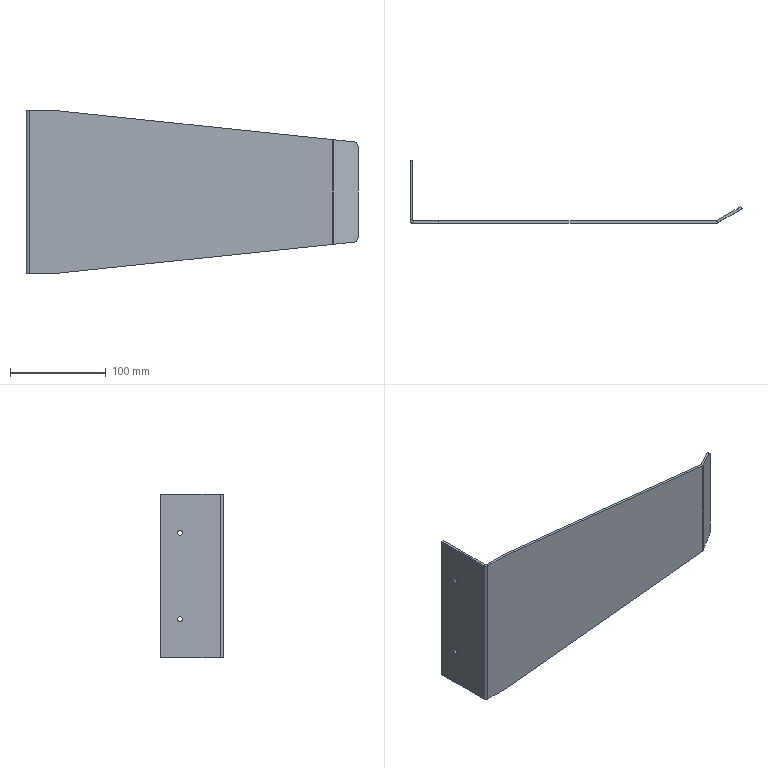Part | SolidWorks | features Fillet 1, FlatPattern 1, HoleWzd 1, ICE 1, MirrorPattern 1, SMBaseFlange 1, SheetMetal 1 | 1 solid | 30 faces | box 345.981 x 65 x 170 mm | volume 147766 mm3 | plane 18 | cylinder 10 | spline 2 | commonest cylinder face diameters 5 x4 1.473 x2 6.473 x2 10 x2
STEP:
#1=CARTESIAN_POINT('',(0.,45.,47.5));
#2=VERTEX_POINT('',#1);
#3=CARTESIAN_POINT('',(0.,45.,42.5));
#4=VERTEX_POINT('',#3);
#5=CARTESIAN_POINT('',(0.,45.,45.));
#6=DIRECTION('',(1.,0.,0.));
#7=DIRECTION('',(0.,0.,-1.));
#8=AXIS2_PLACEMENT_3D('',#5,#6,#7);
#9=CIRCLE('',#8,2.5);
#10=EDGE_CURVE('',#2,#4,#9,.T.);
#11=ORIENTED_EDGE('',*,*,#10,.F.);
#12=CARTESIAN_POINT('',(2.5,45.,47.5));
#13=VERTEX_POINT('',#12);
#14=CARTESIAN_POINT('',(2.5,45.,47.5));
#15=DIRECTION('',(1.,0.,0.));
#16=VECTOR('',#15,1000.);
#17=LINE('',#14,#16);
#18=EDGE_CURVE('',#2,#13,#17,.T.);
#19=ORIENTED_EDGE('',*,*,#18,.T.);
#20=CARTESIAN_POINT('',(2.5,45.,42.5));
#21=VERTEX_POINT('',#20);
#22=CARTESIAN_POINT('',(2.5,45.,45.));
#23=DIRECTION('',(1.,0.,0.));
#24=DIRECTION('',(0.,0.,-1.));
#25=AXIS2_PLACEMENT_3D('',#22,#23,#24);
#26=CIRCLE('',#25,2.5);
#27=EDGE_CURVE('',#13,#21,#26,.T.);
#28=ORIENTED_EDGE('',*,*,#27,.T.);
#29=CARTESIAN_POINT('',(2.5,45.,42.5));
#30=DIRECTION('',(1.,0.,0.));
#31=VECTOR('',#30,1000.);
#32=LINE('',#29,#31);
#33=EDGE_CURVE('',#4,#21,#32,.T.);
#34=ORIENTED_EDGE('',*,*,#33,.F.);
#35=EDGE_LOOP('',(#11,#19,#28,#34));
#36=FACE_OUTER_BOUND('',#35,.T.);
#37=CARTESIAN_POINT('',(2.5,45.,45.));
#38=DIRECTION('',(1.,0.,0.));
#39=DIRECTION('',(0.,0.,-1.));
#40=AXIS2_PLACEMENT_3D('',#37,#38,#39);
#41=CYLINDRICAL_SURFACE('',#40,2.5);
#42=ADVANCED_FACE('',(#36),#41,.F.);
#43=CARTESIAN_POINT('',(0.,45.,-42.5));
#44=VERTEX_POINT('',#43);
#45=CARTESIAN_POINT('',(0.,45.,-47.5));
#46=VERTEX_POINT('',#45);
#47=CARTESIAN_POINT('',(0.,45.,-45.));
#48=DIRECTION('',(1.,0.,0.));
#49=DIRECTION('',(0.,0.,-1.));
#50=AXIS2_PLACEMENT_3D('',#47,#48,#49);
#51=CIRCLE('',#50,2.5);
#52=EDGE_CURVE('',#44,#46,#51,.T.);
#53=ORIENTED_EDGE('',*,*,#52,.F.);
#54=CARTESIAN_POINT('',(2.5,45.,-42.5));
#55=VERTEX_POINT('',#54);
#56=CARTESIAN_POINT('',(2.5,45.,-42.5));
#57=DIRECTION('',(1.,0.,0.));
#58=VECTOR('',#57,1000.);
#59=LINE('',#56,#58);
#60=EDGE_CURVE('',#44,#55,#59,.T.);
#61=ORIENTED_EDGE('',*,*,#60,.T.);
#62=CARTESIAN_POINT('',(2.5,45.,-47.5));
#63=VERTEX_POINT('',#62);
#64=CARTESIAN_POINT('',(2.5,45.,-45.));
#65=DIRECTION('',(1.,0.,0.));
#66=DIRECTION('',(0.,0.,-1.));
#67=AXIS2_PLACEMENT_3D('',#64,#65,#66);
#68=CIRCLE('',#67,2.5);
#69=EDGE_CURVE('',#55,#63,#68,.T.);
#70=ORIENTED_EDGE('',*,*,#69,.T.);
#71=CARTESIAN_POINT('',(2.5,45.,-47.5));
#72=DIRECTION('',(1.,0.,0.));
#73=VECTOR('',#72,1000.);
#74=LINE('',#71,#73);
#75=EDGE_CURVE('',#46,#63,#74,.T.);
#76=ORIENTED_EDGE('',*,*,#75,.F.);
#77=EDGE_LOOP('',(#53,#61,#70,#76));
#78=FACE_OUTER_BOUND('',#77,.T.);
#79=CARTESIAN_POINT('',(2.5,45.,-45.));
#80=DIRECTION('',(1.,0.,0.));
#81=DIRECTION('',(0.,0.,-1.));
#82=AXIS2_PLACEMENT_3D('',#79,#80,#81);
#83=CYLINDRICAL_SURFACE('',#82,2.5);
#84=ADVANCED_FACE('',(#78),#83,.F.);
#85=CARTESIAN_POINT('',(320.751,0.4336,-54.441));
#86=VERTEX_POINT('',#85);
#87=CARTESIAN_POINT('',(342.043,12.727,-52.203));
#88=VERTEX_POINT('',#87);
#89=CARTESIAN_POINT('',(330.908,6.298,-53.373));
#90=DIRECTION('',(0.8625,0.4979,0.09065));
#91=VECTOR('',#90,1000.);
#92=LINE('',#89,#91);
#93=EDGE_CURVE('',#86,#88,#92,.T.);
#94=ORIENTED_EDGE('',*,*,#93,.T.);
#95=CARTESIAN_POINT('',(345.981,15.,-47.224));
#96=VERTEX_POINT('',#95);
#97=CARTESIAN_POINT('',(341.651,12.5,-47.224));
#98=DIRECTION('',(0.5,-0.866,0.));
#99=DIRECTION('',(-0.866,-0.5,0.));
#100=AXIS2_PLACEMENT_3D('',#97,#98,#99);
#101=CIRCLE('',#100,5.);
#102=EDGE_CURVE('',#88,#96,#101,.T.);
#103=ORIENTED_EDGE('',*,*,#102,.T.);
#104=CARTESIAN_POINT('',(345.981,15.,47.224));
#105=VERTEX_POINT('',#104);
#106=CARTESIAN_POINT('',(345.981,15.,85.));
#107=DIRECTION('',(0.,0.,-1.));
#108=VECTOR('',#107,1000.);
#109=LINE('',#106,#108);
#110=EDGE_CURVE('',#105,#96,#109,.T.);
#111=ORIENTED_EDGE('',*,*,#110,.F.);
#112=CARTESIAN_POINT('',(342.043,12.727,52.203));
#113=VERTEX_POINT('',#112);
#114=CARTESIAN_POINT('',(341.651,12.5,47.224));
#115=DIRECTION('',(0.5,-0.866,0.));
#116=DIRECTION('',(-0.866,-0.5,0.));
#117=AXIS2_PLACEMENT_3D('',#114,#115,#116);
#118=CIRCLE('',#117,5.);
#119=EDGE_CURVE('',#105,#113,#118,.T.);
#120=ORIENTED_EDGE('',*,*,#119,.T.);
#121=CARTESIAN_POINT('',(320.751,0.4336,54.441));
#122=VERTEX_POINT('',#121);
#123=CARTESIAN_POINT('',(317.617,-1.376,54.77));
#124=DIRECTION('',(0.8625,0.4979,-0.09065));
#125=VECTOR('',#124,1000.);
#126=LINE('',#123,#125);
#127=EDGE_CURVE('',#122,#113,#126,.T.);
#128=ORIENTED_EDGE('',*,*,#127,.F.);
#129=CARTESIAN_POINT('',(320.751,0.4336,85.));
#130=DIRECTION('',(0.,0.,-1.));
#131=VECTOR('',#130,1000.);
#132=LINE('',#129,#131);
#133=EDGE_CURVE('',#122,#86,#132,.T.);
#134=ORIENTED_EDGE('',*,*,#133,.T.);
#135=EDGE_LOOP('',(#94,#103,#111,#120,#128,#134));
#136=FACE_OUTER_BOUND('',#135,.T.);
#137=CARTESIAN_POINT('',(320.,0.,85.));
#138=DIRECTION('',(-0.5,0.866,0.));
#139=DIRECTION('',(-0.866,-0.5,0.));
#140=AXIS2_PLACEMENT_3D('',#137,#138,#139);
#141=PLANE('',#140);
#142=ADVANCED_FACE('',(#136),#141,.F.);
#143=ORIENTED_EDGE('',*,*,#110,.T.);
#144=CARTESIAN_POINT('',(344.731,17.165,-47.224));
#145=VERTEX_POINT('',#144);
#146=CARTESIAN_POINT('',(344.731,17.165,-47.224));
#147=DIRECTION('',(-0.5,0.866,0.));
#148=VECTOR('',#147,1000.);
#149=LINE('',#146,#148);
#150=EDGE_CURVE('',#96,#145,#149,.T.);
#151=ORIENTED_EDGE('',*,*,#150,.T.);
#152=CARTESIAN_POINT('',(344.731,17.165,47.224));
#153=VERTEX_POINT('',#152);
#154=CARTESIAN_POINT('',(344.731,17.165,85.));
#155=DIRECTION('',(0.,0.,-1.));
#156=VECTOR('',#155,1000.);
#157=LINE('',#154,#156);
#158=EDGE_CURVE('',#153,#145,#157,.T.);
#159=ORIENTED_EDGE('',*,*,#158,.F.);
#160=CARTESIAN_POINT('',(344.731,17.165,47.224));
#161=DIRECTION('',(0.5,-0.866,0.));
#162=VECTOR('',#161,1000.);
#163=LINE('',#160,#162);
#164=EDGE_CURVE('',#153,#105,#163,.T.);
#165=ORIENTED_EDGE('',*,*,#164,.T.);
#166=EDGE_LOOP('',(#143,#151,#159,#165));
#167=FACE_OUTER_BOUND('',#166,.T.);
#168=CARTESIAN_POINT('',(344.731,17.165,85.));
#169=DIRECTION('',(0.866,0.5,0.));
#170=DIRECTION('',(-0.5,0.866,0.));
#171=AXIS2_PLACEMENT_3D('',#168,#169,#170);
#172=PLANE('',#171);
#173=ADVANCED_FACE('',(#167),#172,.T.);
#174=ORIENTED_EDGE('',*,*,#158,.T.);
#175=CARTESIAN_POINT('',(340.793,14.892,-52.203));
#176=VERTEX_POINT('',#175);
#177=CARTESIAN_POINT('',(340.401,14.665,-47.224));
#178=DIRECTION('',(-0.5,0.866,0.));
#179=DIRECTION('',(-0.866,-0.5,0.));
#180=AXIS2_PLACEMENT_3D('',#177,#178,#179);
#181=CIRCLE('',#180,5.);
#182=EDGE_CURVE('',#145,#176,#181,.T.);
#183=ORIENTED_EDGE('',*,*,#182,.T.);
#184=CARTESIAN_POINT('',(319.501,2.599,-54.441));
#185=VERTEX_POINT('',#184);
#186=CARTESIAN_POINT('',(329.658,8.463,-53.373));
#187=DIRECTION('',(0.8625,0.4979,0.09065));
#188=VECTOR('',#187,1000.);
#189=LINE('',#186,#188);
#190=EDGE_CURVE('',#185,#176,#189,.T.);
#191=ORIENTED_EDGE('',*,*,#190,.F.);
#192=CARTESIAN_POINT('',(319.501,2.599,54.441));
#193=VERTEX_POINT('',#192);
#194=CARTESIAN_POINT('',(319.501,2.599,85.));
#195=DIRECTION('',(0.,0.,-1.));
#196=VECTOR('',#195,1000.);
#197=LINE('',#194,#196);
#198=EDGE_CURVE('',#193,#185,#197,.T.);
#199=ORIENTED_EDGE('',*,*,#198,.F.);
#200=CARTESIAN_POINT('',(340.793,14.892,52.203));
#201=VERTEX_POINT('',#200);
#202=CARTESIAN_POINT('',(316.367,0.7893,54.77));
#203=DIRECTION('',(0.8625,0.4979,-0.09065));
#204=VECTOR('',#203,1000.);
#205=LINE('',#202,#204);
#206=EDGE_CURVE('',#193,#201,#205,.T.);
#207=ORIENTED_EDGE('',*,*,#206,.T.);
#208=CARTESIAN_POINT('',(340.401,14.665,47.224));
#209=DIRECTION('',(-0.5,0.866,0.));
#210=DIRECTION('',(-0.866,-0.5,0.));
#211=AXIS2_PLACEMENT_3D('',#208,#209,#210);
#212=CIRCLE('',#211,5.);
#213=EDGE_CURVE('',#201,#153,#212,.T.);
#214=ORIENTED_EDGE('',*,*,#213,.T.);
#215=EDGE_LOOP('',(#174,#183,#191,#199,#207,#214));
#216=FACE_OUTER_BOUND('',#215,.T.);
#217=CARTESIAN_POINT('',(318.75,2.165,85.));
#218=DIRECTION('',(-0.5,0.866,0.));
#219=DIRECTION('',(-0.866,-0.5,0.));
#220=AXIS2_PLACEMENT_3D('',#217,#218,#219);
#221=PLANE('',#220);
#222=ADVANCED_FACE('',(#216),#221,.T.);
#223=CARTESIAN_POINT('',(319.133,2.5,54.611));
#224=VERTEX_POINT('',#223);
#225=CARTESIAN_POINT('',(319.133,2.5,-54.611));
#226=VERTEX_POINT('',#225);
#227=CARTESIAN_POINT('',(319.133,2.5,85.));
#228=DIRECTION('',(0.,0.,-1.));
#229=VECTOR('',#228,1000.);
#230=LINE('',#227,#229);
#231=EDGE_CURVE('',#224,#226,#230,.T.);
#232=ORIENTED_EDGE('',*,*,#231,.F.);
#233=CARTESIAN_POINT('',(319.133,2.5,54.611));
#234=CARTESIAN_POINT('',(319.263,2.5,54.551));
#235=CARTESIAN_POINT('',(319.388,2.534,54.493));
#236=CARTESIAN_POINT('',(319.501,2.599,54.441));
#237=(BOUNDED_CURVE()B_SPLINE_CURVE(3,(#233,#234,#235,#236),.UNSPECIFIED.,.F.,.T.)B_SPLINE_CURVE_WITH_KNOTS((4,4),(4.712,5.236),.UNSPECIFIED.)CURVE()GEOMETRIC_REPRESENTATION_ITEM()RATIONAL_B_SPLINE_CURVE((1.,0.9773,0.9773,1.))REPRESENTATION_ITEM(''));
#238=EDGE_CURVE('',#224,#193,#237,.T.);
#239=ORIENTED_EDGE('',*,*,#238,.T.);
#240=ORIENTED_EDGE('',*,*,#198,.T.);
#241=CARTESIAN_POINT('',(319.133,2.5,-54.611));
#242=CARTESIAN_POINT('',(319.263,2.5,-54.551));
#243=CARTESIAN_POINT('',(319.388,2.534,-54.493));
#244=CARTESIAN_POINT('',(319.501,2.599,-54.441));
#245=(BOUNDED_CURVE()B_SPLINE_CURVE(3,(#241,#242,#243,#244),.UNSPECIFIED.,.F.,.T.)B_SPLINE_CURVE_WITH_KNOTS((4,4),(1.571,2.094),.UNSPECIFIED.)CURVE()GEOMETRIC_REPRESENTATION_ITEM()RATIONAL_B_SPLINE_CURVE((1.,0.9773,0.9773,1.))REPRESENTATION_ITEM(''));
#246=EDGE_CURVE('',#226,#185,#245,.T.);
#247=ORIENTED_EDGE('',*,*,#246,.F.);
#248=EDGE_LOOP('',(#232,#239,#240,#247));
#249=FACE_OUTER_BOUND('',#248,.T.);
#250=CARTESIAN_POINT('',(319.133,3.237,85.));
#251=DIRECTION('',(0.,0.,-1.));
#252=DIRECTION('',(-1.,0.,0.));
#253=AXIS2_PLACEMENT_3D('',#250,#251,#252);
#254=CYLINDRICAL_SURFACE('',#253,0.7366);
#255=ADVANCED_FACE('',(#249),#254,.F.);
#256=CARTESIAN_POINT('',(3.237,2.5,85.));
#257=VERTEX_POINT('',#256);
#258=CARTESIAN_POINT('',(30.,2.5,85.));
#259=VERTEX_POINT('',#258);
#260=CARTESIAN_POINT('',(0.,2.5,85.));
#261=DIRECTION('',(1.,0.,0.));
#262=VECTOR('',#261,1000.);
#263=LINE('',#260,#262);
#264=EDGE_CURVE('',#257,#259,#263,.T.);
#265=ORIENTED_EDGE('',*,*,#264,.T.);
#266=CARTESIAN_POINT('',(0.3278,2.5,88.119));
#267=DIRECTION('',(0.9945,0.,-0.1045));
#268=VECTOR('',#267,1000.);
#269=LINE('',#266,#268);
#270=EDGE_CURVE('',#259,#224,#269,.T.);
#271=ORIENTED_EDGE('',*,*,#270,.T.);
#272=ORIENTED_EDGE('',*,*,#231,.T.);
#273=CARTESIAN_POINT('',(30.,2.5,-85.));
#274=VERTEX_POINT('',#273);
#275=CARTESIAN_POINT('',(18.,2.5,-86.261));
#276=DIRECTION('',(0.9945,0.,0.1045));
#277=VECTOR('',#276,1000.);
#278=LINE('',#275,#277);
#279=EDGE_CURVE('',#274,#226,#278,.T.);
#280=ORIENTED_EDGE('',*,*,#279,.F.);
#281=CARTESIAN_POINT('',(3.237,2.5,-85.));
#282=VERTEX_POINT('',#281);
#283=CARTESIAN_POINT('',(0.,2.5,-85.));
#284=DIRECTION('',(1.,0.,0.));
#285=VECTOR('',#284,1000.);
#286=LINE('',#283,#285);
#287=EDGE_CURVE('',#282,#274,#286,.T.);
#288=ORIENTED_EDGE('',*,*,#287,.F.);
#289=CARTESIAN_POINT('',(3.237,2.5,85.));
#290=DIRECTION('',(0.,0.,-1.));
#291=VECTOR('',#290,1000.);
#292=LINE('',#289,#291);
#293=EDGE_CURVE('',#257,#282,#292,.T.);
#294=ORIENTED_EDGE('',*,*,#293,.F.);
#295=EDGE_LOOP('',(#265,#271,#272,#280,#288,#294));
#296=FACE_OUTER_BOUND('',#295,.T.);
#297=CARTESIAN_POINT('',(0.,2.5,85.));
#298=DIRECTION('',(0.,1.,0.));
#299=DIRECTION('',(0.,0.,1.));
#300=AXIS2_PLACEMENT_3D('',#297,#298,#299);
#301=PLANE('',#300);
#302=ADVANCED_FACE('',(#296),#301,.T.);
#303=CARTESIAN_POINT('',(30.,0.,85.));
#304=VERTEX_POINT('',#303);
#305=CARTESIAN_POINT('',(319.133,0.,54.611));
#306=VERTEX_POINT('',#305);
#307=CARTESIAN_POINT('',(0.3278,0.,88.119));
#308=DIRECTION('',(0.9945,0.,-0.1045));
#309=VECTOR('',#308,1000.);
#310=LINE('',#307,#309);
#311=EDGE_CURVE('',#304,#306,#310,.T.);
#312=ORIENTED_EDGE('',*,*,#311,.F.);
#313=CARTESIAN_POINT('',(3.237,0.,85.));
#314=VERTEX_POINT('',#313);
#315=CARTESIAN_POINT('',(0.,0.,85.));
#316=DIRECTION('',(1.,0.,0.));
#317=VECTOR('',#316,1000.);
#318=LINE('',#315,#317);
#319=EDGE_CURVE('',#314,#304,#318,.T.);
#320=ORIENTED_EDGE('',*,*,#319,.F.);
#321=CARTESIAN_POINT('',(3.237,0.,-85.));
#322=VERTEX_POINT('',#321);
#323=CARTESIAN_POINT('',(3.237,0.,85.));
#324=DIRECTION('',(0.,0.,-1.));
#325=VECTOR('',#324,1000.);
#326=LINE('',#323,#325);
#327=EDGE_CURVE('',#314,#322,#326,.T.);
#328=ORIENTED_EDGE('',*,*,#327,.T.);
#329=CARTESIAN_POINT('',(30.,0.,-85.));
#330=VERTEX_POINT('',#329);
#331=CARTESIAN_POINT('',(0.,0.,-85.));
#332=DIRECTION('',(1.,0.,0.));
#333=VECTOR('',#332,1000.);
#334=LINE('',#331,#333);
#335=EDGE_CURVE('',#322,#330,#334,.T.);
#336=ORIENTED_EDGE('',*,*,#335,.T.);
#337=CARTESIAN_POINT('',(319.133,0.,-54.611));
#338=VERTEX_POINT('',#337);
#339=CARTESIAN_POINT('',(18.,0.,-86.261));
#340=DIRECTION('',(0.9945,0.,0.1045));
#341=VECTOR('',#340,1000.);
#342=LINE('',#339,#341);
#343=EDGE_CURVE('',#330,#338,#342,.T.);
#344=ORIENTED_EDGE('',*,*,#343,.T.);
#345=CARTESIAN_POINT('',(319.133,0.,85.));
#346=DIRECTION('',(0.,0.,-1.));
#347=VECTOR('',#346,1000.);
#348=LINE('',#345,#347);
#349=EDGE_CURVE('',#306,#338,#348,.T.);
#350=ORIENTED_EDGE('',*,*,#349,.F.);
#351=EDGE_LOOP('',(#312,#320,#328,#336,#344,#350));
#352=FACE_OUTER_BOUND('',#351,.T.);
#353=CARTESIAN_POINT('',(0.,0.,85.));
#354=DIRECTION('',(0.,1.,0.));
#355=DIRECTION('',(0.,0.,1.));
#356=AXIS2_PLACEMENT_3D('',#353,#354,#355);
#357=PLANE('',#356);
#358=ADVANCED_FACE('',(#352),#357,.F.);
#359=CARTESIAN_POINT('',(319.133,0.,54.611));
#360=CARTESIAN_POINT('',(319.704,0.,54.551));
#361=CARTESIAN_POINT('',(320.256,0.1479,54.493));
#362=CARTESIAN_POINT('',(320.751,0.4336,54.441));
#363=(BOUNDED_CURVE()B_SPLINE_CURVE(3,(#359,#360,#361,#362),.UNSPECIFIED.,.F.,.F.)B_SPLINE_CURVE_WITH_KNOTS((4,4),(4.712,5.236),.UNSPECIFIED.)CURVE()GEOMETRIC_REPRESENTATION_ITEM()RATIONAL_B_SPLINE_CURVE((1.,0.9773,0.9773,1.))REPRESENTATION_ITEM(''));
#364=EDGE_CURVE('',#306,#122,#363,.T.);
#365=ORIENTED_EDGE('',*,*,#364,.F.);
#366=ORIENTED_EDGE('',*,*,#349,.T.);
#367=CARTESIAN_POINT('',(319.133,0.,-54.611));
#368=CARTESIAN_POINT('',(319.704,0.,-54.551));
#369=CARTESIAN_POINT('',(320.256,0.1479,-54.493));
#370=CARTESIAN_POINT('',(320.751,0.4336,-54.441));
#371=(BOUNDED_CURVE()B_SPLINE_CURVE(3,(#367,#368,#369,#370),.UNSPECIFIED.,.F.,.F.)B_SPLINE_CURVE_WITH_KNOTS((4,4),(1.571,2.094),.UNSPECIFIED.)CURVE()GEOMETRIC_REPRESENTATION_ITEM()RATIONAL_B_SPLINE_CURVE((1.,0.9773,0.9773,1.))REPRESENTATION_ITEM(''));
#372=EDGE_CURVE('',#338,#86,#371,.T.);
#373=ORIENTED_EDGE('',*,*,#372,.T.);
#374=ORIENTED_EDGE('',*,*,#133,.F.);
#375=EDGE_LOOP('',(#365,#366,#373,#374));
#376=FACE_OUTER_BOUND('',#375,.T.);
#377=CARTESIAN_POINT('',(319.133,3.237,85.));
#378=DIRECTION('',(0.,0.,-1.));
#379=DIRECTION('',(-1.,0.,0.));
#380=AXIS2_PLACEMENT_3D('',#377,#378,#379);
#381=CYLINDRICAL_SURFACE('',#380,3.237);
#382=ADVANCED_FACE('',(#376),#381,.T.);
#383=ORIENTED_EDGE('',*,*,#319,.T.);
#384=CARTESIAN_POINT('',(30.,2.5,85.));
#385=DIRECTION('',(0.,-1.,0.));
#386=VECTOR('',#385,1000.);
#387=LINE('',#384,#386);
#388=EDGE_CURVE('',#259,#304,#387,.T.);
#389=ORIENTED_EDGE('',*,*,#388,.F.);
#390=ORIENTED_EDGE('',*,*,#264,.F.);
#391=CARTESIAN_POINT('',(3.237,2.5,85.));
#392=DIRECTION('',(0.,-1.,0.));
#393=VECTOR('',#392,1000.);
#394=LINE('',#391,#393);
#395=EDGE_CURVE('',#257,#314,#394,.T.);
#396=ORIENTED_EDGE('',*,*,#395,.T.);
#397=EDGE_LOOP('',(#383,#389,#390,#396));
#398=FACE_OUTER_BOUND('',#397,.T.);
#399=CARTESIAN_POINT('',(319.501,2.599,85.));
#400=DIRECTION('',(0.,0.,1.));
#401=DIRECTION('',(1.,0.,0.));
#402=AXIS2_PLACEMENT_3D('',#399,#400,#401);
#403=PLANE('',#402);
#404=ADVANCED_FACE('',(#398),#403,.T.);
#405=ORIENTED_EDGE('',*,*,#287,.T.);
#406=CARTESIAN_POINT('',(30.,2.5,-85.));
#407=DIRECTION('',(0.,-1.,0.));
#408=VECTOR('',#407,1000.);
#409=LINE('',#406,#408);
#410=EDGE_CURVE('',#274,#330,#409,.T.);
#411=ORIENTED_EDGE('',*,*,#410,.T.);
#412=ORIENTED_EDGE('',*,*,#335,.F.);
#413=CARTESIAN_POINT('',(3.237,0.,-85.));
#414=DIRECTION('',(0.,1.,0.));
#415=VECTOR('',#414,1000.);
#416=LINE('',#413,#415);
#417=EDGE_CURVE('',#322,#282,#416,.T.);
#418=ORIENTED_EDGE('',*,*,#417,.T.);
#419=EDGE_LOOP('',(#405,#411,#412,#418));
#420=FACE_OUTER_BOUND('',#419,.T.);
#421=CARTESIAN_POINT('',(2.5,3.237,-85.));
#422=DIRECTION('',(0.,0.,-1.));
#423=DIRECTION('',(-1.,0.,0.));
#424=AXIS2_PLACEMENT_3D('',#421,#422,#423);
#425=PLANE('',#424);
#426=ADVANCED_FACE('',(#420),#425,.T.);
#427=CARTESIAN_POINT('',(0.,3.237,85.));
#428=VERTEX_POINT('',#427);
#429=CARTESIAN_POINT('',(2.5,3.237,85.));
#430=VERTEX_POINT('',#429);
#431=CARTESIAN_POINT('',(0.,3.237,85.));
#432=DIRECTION('',(1.,0.,0.));
#433=VECTOR('',#432,1000.);
#434=LINE('',#431,#433);
#435=EDGE_CURVE('',#428,#430,#434,.T.);
#436=ORIENTED_EDGE('',*,*,#435,.F.);
#437=CARTESIAN_POINT('',(3.237,3.237,85.));
#438=DIRECTION('',(0.,0.,1.));
#439=DIRECTION('',(-1.,0.,0.));
#440=AXIS2_PLACEMENT_3D('',#437,#438,#439);
#441=CIRCLE('',#440,3.237);
#442=EDGE_CURVE('',#428,#314,#441,.T.);
#443=ORIENTED_EDGE('',*,*,#442,.T.);
#444=ORIENTED_EDGE('',*,*,#395,.F.);
#445=CARTESIAN_POINT('',(3.237,3.237,85.));
#446=DIRECTION('',(0.,0.,1.));
#447=DIRECTION('',(1.,0.,0.));
#448=AXIS2_PLACEMENT_3D('',#445,#446,#447);
#449=CIRCLE('',#448,0.7366);
#450=EDGE_CURVE('',#430,#257,#449,.T.);
#451=ORIENTED_EDGE('',*,*,#450,.F.);
#452=EDGE_LOOP('',(#436,#443,#444,#451));
#453=FACE_OUTER_BOUND('',#452,.T.);
#454=CARTESIAN_POINT('',(0.,3.237,85.));
#455=DIRECTION('',(0.,0.,1.));
#456=DIRECTION('',(1.,0.,0.));
#457=AXIS2_PLACEMENT_3D('',#454,#455,#456);
#458=PLANE('',#457);
#459=ADVANCED_FACE('',(#453),#458,.T.);
#460=CARTESIAN_POINT('',(0.,65.,85.));
#461=VERTEX_POINT('',#460);
#462=CARTESIAN_POINT('',(0.,65.,85.));
#463=DIRECTION('',(0.,-1.,0.));
#464=VECTOR('',#463,1000.);
#465=LINE('',#462,#464);
#466=EDGE_CURVE('',#461,#428,#465,.T.);
#467=ORIENTED_EDGE('',*,*,#466,.T.);
#468=ORIENTED_EDGE('',*,*,#435,.T.);
#469=CARTESIAN_POINT('',(2.5,65.,85.));
#470=VERTEX_POINT('',#469);
#471=CARTESIAN_POINT('',(2.5,65.,85.));
#472=DIRECTION('',(0.,-1.,0.));
#473=VECTOR('',#472,1000.);
#474=LINE('',#471,#473);
#475=EDGE_CURVE('',#470,#430,#474,.T.);
#476=ORIENTED_EDGE('',*,*,#475,.F.);
#477=CARTESIAN_POINT('',(0.,65.,85.));
#478=DIRECTION('',(1.,0.,0.));
#479=VECTOR('',#478,1000.);
#480=LINE('',#477,#479);
#481=EDGE_CURVE('',#461,#470,#480,.T.);
#482=ORIENTED_EDGE('',*,*,#481,.F.);
#483=EDGE_LOOP('',(#467,#468,#476,#482));
#484=FACE_OUTER_BOUND('',#483,.T.);
#485=CARTESIAN_POINT('',(3.237,2.5,85.));
#486=DIRECTION('',(0.,0.,1.));
#487=DIRECTION('',(1.,0.,0.));
#488=AXIS2_PLACEMENT_3D('',#485,#486,#487);
#489=PLANE('',#488);
#490=ADVANCED_FACE('',(#484),#489,.T.);
#491=ORIENTED_EDGE('',*,*,#417,.F.);
#492=CARTESIAN_POINT('',(0.,3.237,-85.));
#493=VERTEX_POINT('',#492);
#494=CARTESIAN_POINT('',(3.237,3.237,-85.));
#495=DIRECTION('',(0.,0.,1.));
#496=DIRECTION('',(-1.,0.,0.));
#497=AXIS2_PLACEMENT_3D('',#494,#495,#496);
#498=CIRCLE('',#497,3.237);
#499=EDGE_CURVE('',#493,#322,#498,.T.);
#500=ORIENTED_EDGE('',*,*,#499,.F.);
#501=CARTESIAN_POINT('',(2.5,3.237,-85.));
#502=VERTEX_POINT('',#501);
#503=CARTESIAN_POINT('',(2.5,3.237,-85.));
#504=DIRECTION('',(-1.,0.,0.));
#505=VECTOR('',#504,1000.);
#506=LINE('',#503,#505);
#507=EDGE_CURVE('',#502,#493,#506,.T.);
#508=ORIENTED_EDGE('',*,*,#507,.F.);
#509=CARTESIAN_POINT('',(3.237,3.237,-85.));
#510=DIRECTION('',(0.,0.,1.));
#511=DIRECTION('',(1.,0.,0.));
#512=AXIS2_PLACEMENT_3D('',#509,#510,#511);
#513=CIRCLE('',#512,0.7366);
#514=EDGE_CURVE('',#502,#282,#513,.T.);
#515=ORIENTED_EDGE('',*,*,#514,.T.);
#516=EDGE_LOOP('',(#491,#500,#508,#515));
#517=FACE_OUTER_BOUND('',#516,.T.);
#518=CARTESIAN_POINT('',(3.237,0.,-85.));
#519=DIRECTION('',(0.,0.,-1.));
#520=DIRECTION('',(-1.,0.,0.));
#521=AXIS2_PLACEMENT_3D('',#518,#519,#520);
#522=PLANE('',#521);
#523=ADVANCED_FACE('',(#517),#522,.T.);
#524=ORIENTED_EDGE('',*,*,#514,.F.);
#525=CARTESIAN_POINT('',(2.5,3.237,85.));
#526=DIRECTION('',(0.,0.,-1.));
#527=VECTOR('',#526,1000.);
#528=LINE('',#525,#527);
#529=EDGE_CURVE('',#430,#502,#528,.T.);
#530=ORIENTED_EDGE('',*,*,#529,.F.);
#531=ORIENTED_EDGE('',*,*,#450,.T.);
#532=ORIENTED_EDGE('',*,*,#293,.T.);
#533=EDGE_LOOP('',(#524,#530,#531,#532));
#534=FACE_OUTER_BOUND('',#533,.T.);
#535=CARTESIAN_POINT('',(3.237,3.237,85.));
#536=DIRECTION('',(0.,0.,-1.));
#537=DIRECTION('',(-1.,0.,0.));
#538=AXIS2_PLACEMENT_3D('',#535,#536,#537);
#539=CYLINDRICAL_SURFACE('',#538,0.7366);
#540=ADVANCED_FACE('',(#534),#539,.F.);
#541=CARTESIAN_POINT('',(2.5,45.,45.));
#542=DIRECTION('',(1.,0.,0.));
#543=DIRECTION('',(0.,0.,-1.));
#544=AXIS2_PLACEMENT_3D('',#541,#542,#543);
#545=CIRCLE('',#544,2.5);
#546=EDGE_CURVE('',#21,#13,#545,.T.);
#547=ORIENTED_EDGE('',*,*,#546,.F.);
#548=ORIENTED_EDGE('',*,*,#27,.F.);
#549=EDGE_LOOP('',(#547,#548));
#550=FACE_BOUND('',#549,.T.);
#551=CARTESIAN_POINT('',(2.5,45.,-45.));
#552=DIRECTION('',(1.,0.,0.));
#553=DIRECTION('',(0.,0.,-1.));
#554=AXIS2_PLACEMENT_3D('',#551,#552,#553);
#555=CIRCLE('',#554,2.5);
#556=EDGE_CURVE('',#63,#55,#555,.T.);
#557=ORIENTED_EDGE('',*,*,#556,.F.);
#558=ORIENTED_EDGE('',*,*,#69,.F.);
#559=EDGE_LOOP('',(#557,#558));
#560=FACE_BOUND('',#559,.T.);
#561=CARTESIAN_POINT('',(2.5,65.,-85.));
#562=VERTEX_POINT('',#561);
#563=CARTESIAN_POINT('',(2.5,65.,-85.));
#564=DIRECTION('',(0.,-1.,0.));
#565=VECTOR('',#564,1000.);
#566=LINE('',#563,#565);
#567=EDGE_CURVE('',#562,#502,#566,.T.);
#568=ORIENTED_EDGE('',*,*,#567,.F.);
#569=CARTESIAN_POINT('',(2.5,65.,85.));
#570=DIRECTION('',(0.,0.,-1.));
#571=VECTOR('',#570,1000.);
#572=LINE('',#569,#571);
#573=EDGE_CURVE('',#470,#562,#572,.T.);
#574=ORIENTED_EDGE('',*,*,#573,.F.);
#575=ORIENTED_EDGE('',*,*,#475,.T.);
#576=ORIENTED_EDGE('',*,*,#529,.T.);
#577=EDGE_LOOP('',(#568,#574,#575,#576));
#578=FACE_OUTER_BOUND('',#577,.T.);
#579=CARTESIAN_POINT('',(2.5,65.,85.));
#580=DIRECTION('',(1.,0.,0.));
#581=DIRECTION('',(0.,0.,-1.));
#582=AXIS2_PLACEMENT_3D('',#579,#580,#581);
#583=PLANE('',#582);
#584=ADVANCED_FACE('',(#550,#560,#578),#583,.T.);
#585=CARTESIAN_POINT('',(0.,65.,-85.));
#586=VERTEX_POINT('',#585);
#587=CARTESIAN_POINT('',(0.,65.,-85.));
#588=DIRECTION('',(1.,0.,0.));
#589=VECTOR('',#588,1000.);
#590=LINE('',#587,#589);
#591=EDGE_CURVE('',#586,#562,#590,.T.);
#592=ORIENTED_EDGE('',*,*,#591,.F.);
#593=CARTESIAN_POINT('',(0.,65.,85.));
#594=DIRECTION('',(0.,0.,-1.));
#595=VECTOR('',#594,1000.);
#596=LINE('',#593,#595);
#597=EDGE_CURVE('',#461,#586,#596,.T.);
#598=ORIENTED_EDGE('',*,*,#597,.F.);
#599=ORIENTED_EDGE('',*,*,#481,.T.);
#600=ORIENTED_EDGE('',*,*,#573,.T.);
#601=EDGE_LOOP('',(#592,#598,#599,#600));
#602=FACE_OUTER_BOUND('',#601,.T.);
#603=CARTESIAN_POINT('',(0.,65.,85.));
#604=DIRECTION('',(0.,1.,0.));
#605=DIRECTION('',(0.,0.,1.));
#606=AXIS2_PLACEMENT_3D('',#603,#604,#605);
#607=PLANE('',#606);
#608=ADVANCED_FACE('',(#602),#607,.T.);
#609=CARTESIAN_POINT('',(0.,45.,45.));
#610=DIRECTION('',(1.,0.,0.));
#611=DIRECTION('',(0.,0.,-1.));
#612=AXIS2_PLACEMENT_3D('',#609,#610,#611);
#613=CIRCLE('',#612,2.5);
#614=EDGE_CURVE('',#4,#2,#613,.T.);
#615=ORIENTED_EDGE('',*,*,#614,.T.);
#616=ORIENTED_EDGE('',*,*,#10,.T.);
#617=EDGE_LOOP('',(#615,#616));
#618=FACE_BOUND('',#617,.T.);
#619=CARTESIAN_POINT('',(0.,45.,-45.));
#620=DIRECTION('',(1.,0.,0.));
#621=DIRECTION('',(0.,0.,-1.));
#622=AXIS2_PLACEMENT_3D('',#619,#620,#621);
#623=CIRCLE('',#622,2.5);
#624=EDGE_CURVE('',#46,#44,#623,.T.);
#625=ORIENTED_EDGE('',*,*,#624,.T.);
#626=ORIENTED_EDGE('',*,*,#52,.T.);
#627=EDGE_LOOP('',(#625,#626));
#628=FACE_BOUND('',#627,.T.);
#629=CARTESIAN_POINT('',(0.,65.,-85.));
#630=DIRECTION('',(0.,-1.,0.));
#631=VECTOR('',#630,1000.);
#632=LINE('',#629,#631);
#633=EDGE_CURVE('',#586,#493,#632,.T.);
#634=ORIENTED_EDGE('',*,*,#633,.T.);
#635=CARTESIAN_POINT('',(0.,3.237,85.));
#636=DIRECTION('',(0.,0.,-1.));
#637=VECTOR('',#636,1000.);
#638=LINE('',#635,#637);
#639=EDGE_CURVE('',#428,#493,#638,.T.);
#640=ORIENTED_EDGE('',*,*,#639,.F.);
#641=ORIENTED_EDGE('',*,*,#466,.F.);
#642=ORIENTED_EDGE('',*,*,#597,.T.);
#643=EDGE_LOOP('',(#634,#640,#641,#642));
#644=FACE_OUTER_BOUND('',#643,.T.);
#645=CARTESIAN_POINT('',(0.,65.,85.));
#646=DIRECTION('',(1.,0.,0.));
#647=DIRECTION('',(0.,0.,-1.));
#648=AXIS2_PLACEMENT_3D('',#645,#646,#647);
#649=PLANE('',#648);
#650=ADVANCED_FACE('',(#618,#628,#644),#649,.F.);
#651=ORIENTED_EDGE('',*,*,#499,.T.);
#652=ORIENTED_EDGE('',*,*,#327,.F.);
#653=ORIENTED_EDGE('',*,*,#442,.F.);
#654=ORIENTED_EDGE('',*,*,#639,.T.);
#655=EDGE_LOOP('',(#651,#652,#653,#654));
#656=FACE_OUTER_BOUND('',#655,.T.);
#657=CARTESIAN_POINT('',(3.237,3.237,85.));
#658=DIRECTION('',(0.,0.,-1.));
#659=DIRECTION('',(-1.,0.,0.));
#660=AXIS2_PLACEMENT_3D('',#657,#658,#659);
#661=CYLINDRICAL_SURFACE('',#660,3.237);
#662=ADVANCED_FACE('',(#656),#661,.T.);
#663=ORIENTED_EDGE('',*,*,#567,.T.);
#664=ORIENTED_EDGE('',*,*,#507,.T.);
#665=ORIENTED_EDGE('',*,*,#633,.F.);
#666=ORIENTED_EDGE('',*,*,#591,.T.);
#667=EDGE_LOOP('',(#663,#664,#665,#666));
#668=FACE_OUTER_BOUND('',#667,.T.);
#669=CARTESIAN_POINT('',(319.133,3.237,-85.));
#670=DIRECTION('',(0.,0.,1.));
#671=DIRECTION('',(1.,0.,0.));
#672=AXIS2_PLACEMENT_3D('',#669,#670,#671);
#673=PLANE('',#672);
#674=ADVANCED_FACE('',(#668),#673,.F.);
#675=ORIENTED_EDGE('',*,*,#279,.T.);
#676=CARTESIAN_POINT('',(319.133,2.5,-54.611));
#677=DIRECTION('',(0.,-1.,0.));
#678=VECTOR('',#677,1000.);
#679=LINE('',#676,#678);
#680=EDGE_CURVE('',#226,#338,#679,.T.);
#681=ORIENTED_EDGE('',*,*,#680,.T.);
#682=ORIENTED_EDGE('',*,*,#343,.F.);
#683=ORIENTED_EDGE('',*,*,#410,.F.);
#684=EDGE_LOOP('',(#675,#681,#682,#683));
#685=FACE_OUTER_BOUND('',#684,.T.);
#686=CARTESIAN_POINT('',(18.,2.5,-86.261));
#687=DIRECTION('',(-0.1045,0.,0.9945));
#688=DIRECTION('',(0.9945,0.,0.1045));
#689=AXIS2_PLACEMENT_3D('',#686,#687,#688);
#690=PLANE('',#689);
#691=ADVANCED_FACE('',(#685),#690,.F.);
#692=ORIENTED_EDGE('',*,*,#190,.T.);
#693=CARTESIAN_POINT('',(342.043,12.727,-52.203));
#694=DIRECTION('',(0.5,-0.866,0.));
#695=VECTOR('',#694,1000.);
#696=LINE('',#693,#695);
#697=EDGE_CURVE('',#176,#88,#696,.T.);
#698=ORIENTED_EDGE('',*,*,#697,.T.);
#699=ORIENTED_EDGE('',*,*,#93,.F.);
#700=CARTESIAN_POINT('',(320.751,0.4336,-54.441));
#701=DIRECTION('',(-0.5,0.866,0.));
#702=VECTOR('',#701,1000.);
#703=LINE('',#700,#702);
#704=EDGE_CURVE('',#86,#185,#703,.T.);
#705=ORIENTED_EDGE('',*,*,#704,.T.);
#706=EDGE_LOOP('',(#692,#698,#699,#705));
#707=FACE_OUTER_BOUND('',#706,.T.);
#708=CARTESIAN_POINT('',(330.908,6.298,-53.373));
#709=DIRECTION('',(-0.0785,-0.04532,0.9959));
#710=DIRECTION('',(0.8625,0.4979,0.09065));
#711=AXIS2_PLACEMENT_3D('',#708,#709,#710);
#712=PLANE('',#711);
#713=ADVANCED_FACE('',(#707),#712,.F.);
#714=ORIENTED_EDGE('',*,*,#704,.F.);
#715=ORIENTED_EDGE('',*,*,#372,.F.);
#716=ORIENTED_EDGE('',*,*,#680,.F.);
#717=ORIENTED_EDGE('',*,*,#246,.T.);
#718=EDGE_LOOP('',(#714,#715,#716,#717));
#719=FACE_OUTER_BOUND('',#718,.T.);
#720=CARTESIAN_POINT('',(318.396,3.237,-54.951));
#721=CARTESIAN_POINT('',(317.563,3.237,-54.951));
#722=CARTESIAN_POINT('',(316.729,3.237,-54.951));
#723=CARTESIAN_POINT('',(315.896,3.237,-54.951));
#724=CARTESIAN_POINT('',(318.396,1.763,-54.951));
#725=CARTESIAN_POINT('',(317.563,0.09673,-54.951));
#726=CARTESIAN_POINT('',(316.729,-1.57,-54.951));
#727=CARTESIAN_POINT('',(315.896,-3.237,-54.951));
#728=CARTESIAN_POINT('',(319.869,1.763,-54.271));
#729=CARTESIAN_POINT('',(320.703,0.09673,-54.271));
#730=CARTESIAN_POINT('',(321.536,-1.57,-54.271));
#731=CARTESIAN_POINT('',(322.369,-3.237,-54.271));
#732=CARTESIAN_POINT('',(319.869,3.237,-54.271));
#733=CARTESIAN_POINT('',(320.703,3.237,-54.271));
#734=CARTESIAN_POINT('',(321.536,3.237,-54.271));
#735=CARTESIAN_POINT('',(322.369,3.237,-54.271));
#736=CARTESIAN_POINT('',(319.869,4.71,-54.271));
#737=CARTESIAN_POINT('',(320.703,6.376,-54.271));
#738=CARTESIAN_POINT('',(321.536,8.043,-54.271));
#739=CARTESIAN_POINT('',(322.369,9.71,-54.271));
#740=CARTESIAN_POINT('',(318.396,4.71,-54.951));
#741=CARTESIAN_POINT('',(317.563,6.376,-54.951));
#742=CARTESIAN_POINT('',(316.729,8.043,-54.951));
#743=CARTESIAN_POINT('',(315.896,9.71,-54.951));
#744=CARTESIAN_POINT('',(318.396,3.237,-54.951));
#745=CARTESIAN_POINT('',(317.563,3.237,-54.951));
#746=CARTESIAN_POINT('',(316.729,3.237,-54.951));
#747=CARTESIAN_POINT('',(315.896,3.237,-54.951));
#748=(BOUNDED_SURFACE()B_SPLINE_SURFACE(3,3,((#720,#721,#722,#723),(#724,#725,#726,#727),(#728,#729,#730,#731),(#732,#733,#734,#735),(#736,#737,#738,#739),(#740,#741,#742,#743),(#744,#745,#746,#747)),.UNSPECIFIED.,.T.,.F.,.F.)B_SPLINE_SURFACE_WITH_KNOTS((4,3,4),(4,4),(0.,0.5,1.),(0.,1.),.UNSPECIFIED.)GEOMETRIC_REPRESENTATION_ITEM()RATIONAL_B_SPLINE_SURFACE(((1.,1.,1.,1.),(0.3333,0.3333,0.3333,0.3333),(0.3333,0.3333,0.3333,0.3333),(1.,1.,1.,1.),(0.3333,0.3333,0.3333,0.3333),(0.3333,0.3333,0.3333,0.3333),(1.,1.,1.,1.)))REPRESENTATION_ITEM('')SURFACE());
#749=ADVANCED_FACE('',(#719),#748,.T.);
#750=CARTESIAN_POINT('',(319.133,2.5,54.611));
#751=DIRECTION('',(0.,-1.,0.));
#752=VECTOR('',#751,1000.);
#753=LINE('',#750,#752);
#754=EDGE_CURVE('',#224,#306,#753,.T.);
#755=ORIENTED_EDGE('',*,*,#754,.F.);
#756=ORIENTED_EDGE('',*,*,#270,.F.);
#757=ORIENTED_EDGE('',*,*,#388,.T.);
#758=ORIENTED_EDGE('',*,*,#311,.T.);
#759=EDGE_LOOP('',(#755,#756,#757,#758));
#760=FACE_OUTER_BOUND('',#759,.T.);
#761=CARTESIAN_POINT('',(0.3278,2.5,88.119));
#762=DIRECTION('',(0.1045,0.,0.9945));
#763=DIRECTION('',(0.9945,0.,-0.1045));
#764=AXIS2_PLACEMENT_3D('',#761,#762,#763);
#765=PLANE('',#764);
#766=ADVANCED_FACE('',(#760),#765,.T.);
#767=ORIENTED_EDGE('',*,*,#127,.T.);
#768=CARTESIAN_POINT('',(342.043,12.727,52.203));
#769=DIRECTION('',(-0.5,0.866,0.));
#770=VECTOR('',#769,1000.);
#771=LINE('',#768,#770);
#772=EDGE_CURVE('',#113,#201,#771,.T.);
#773=ORIENTED_EDGE('',*,*,#772,.T.);
#774=ORIENTED_EDGE('',*,*,#206,.F.);
#775=CARTESIAN_POINT('',(320.751,0.4336,54.441));
#776=DIRECTION('',(-0.5,0.866,0.));
#777=VECTOR('',#776,1000.);
#778=LINE('',#775,#777);
#779=EDGE_CURVE('',#122,#193,#778,.T.);
#780=ORIENTED_EDGE('',*,*,#779,.F.);
#781=EDGE_LOOP('',(#767,#773,#774,#780));
#782=FACE_OUTER_BOUND('',#781,.T.);
#783=CARTESIAN_POINT('',(317.617,-1.376,54.77));
#784=DIRECTION('',(0.0785,0.04532,0.9959));
#785=DIRECTION('',(0.8625,0.4979,-0.09065));
#786=AXIS2_PLACEMENT_3D('',#783,#784,#785);
#787=PLANE('',#786);
#788=ADVANCED_FACE('',(#782),#787,.T.);
#789=ORIENTED_EDGE('',*,*,#364,.T.);
#790=ORIENTED_EDGE('',*,*,#779,.T.);
#791=ORIENTED_EDGE('',*,*,#238,.F.);
#792=ORIENTED_EDGE('',*,*,#754,.T.);
#793=EDGE_LOOP('',(#789,#790,#791,#792));
#794=FACE_OUTER_BOUND('',#793,.T.);
#795=CARTESIAN_POINT('',(319.869,3.237,54.271));
#796=CARTESIAN_POINT('',(320.703,3.237,54.271));
#797=CARTESIAN_POINT('',(321.536,3.237,54.271));
#798=CARTESIAN_POINT('',(322.369,3.237,54.271));
#799=CARTESIAN_POINT('',(319.869,4.71,54.271));
#800=CARTESIAN_POINT('',(320.703,6.376,54.271));
#801=CARTESIAN_POINT('',(321.536,8.043,54.271));
#802=CARTESIAN_POINT('',(322.369,9.71,54.271));
#803=CARTESIAN_POINT('',(318.396,4.71,54.951));
#804=CARTESIAN_POINT('',(317.563,6.376,54.951));
#805=CARTESIAN_POINT('',(316.729,8.043,54.951));
#806=CARTESIAN_POINT('',(315.896,9.71,54.951));
#807=CARTESIAN_POINT('',(318.396,3.237,54.951));
#808=CARTESIAN_POINT('',(317.563,3.237,54.951));
#809=CARTESIAN_POINT('',(316.729,3.237,54.951));
#810=CARTESIAN_POINT('',(315.896,3.237,54.951));
#811=CARTESIAN_POINT('',(318.396,1.763,54.951));
#812=CARTESIAN_POINT('',(317.563,0.09673,54.951));
#813=CARTESIAN_POINT('',(316.729,-1.57,54.951));
#814=CARTESIAN_POINT('',(315.896,-3.237,54.951));
#815=CARTESIAN_POINT('',(319.869,1.763,54.271));
#816=CARTESIAN_POINT('',(320.703,0.09673,54.271));
#817=CARTESIAN_POINT('',(321.536,-1.57,54.271));
#818=CARTESIAN_POINT('',(322.369,-3.237,54.271));
#819=CARTESIAN_POINT('',(319.869,3.237,54.271));
#820=CARTESIAN_POINT('',(320.703,3.237,54.271));
#821=CARTESIAN_POINT('',(321.536,3.237,54.271));
#822=CARTESIAN_POINT('',(322.369,3.237,54.271));
#823=(BOUNDED_SURFACE()B_SPLINE_SURFACE(3,3,((#795,#796,#797,#798),(#799,#800,#801,#802),(#803,#804,#805,#806),(#807,#808,#809,#810),(#811,#812,#813,#814),(#815,#816,#817,#818),(#819,#820,#821,#822)),.UNSPECIFIED.,.T.,.F.,.F.)B_SPLINE_SURFACE_WITH_KNOTS((4,3,4),(4,4),(0.,0.5,1.),(0.,1.),.UNSPECIFIED.)GEOMETRIC_REPRESENTATION_ITEM()RATIONAL_B_SPLINE_SURFACE(((1.,1.,1.,1.),(0.3333,0.3333,0.3333,0.3333),(0.3333,0.3333,0.3333,0.3333),(1.,1.,1.,1.),(0.3333,0.3333,0.3333,0.3333),(0.3333,0.3333,0.3333,0.3333),(1.,1.,1.,1.)))REPRESENTATION_ITEM('')SURFACE());
#824=ADVANCED_FACE('',(#794),#823,.F.);
#825=ORIENTED_EDGE('',*,*,#102,.F.);
#826=ORIENTED_EDGE('',*,*,#697,.F.);
#827=ORIENTED_EDGE('',*,*,#182,.F.);
#828=ORIENTED_EDGE('',*,*,#150,.F.);
#829=EDGE_LOOP('',(#825,#826,#827,#828));
#830=FACE_OUTER_BOUND('',#829,.T.);
#831=CARTESIAN_POINT('',(340.401,14.665,-47.224));
#832=DIRECTION('',(0.5,-0.866,0.));
#833=DIRECTION('',(0.866,0.5,0.));
#834=AXIS2_PLACEMENT_3D('',#831,#832,#833);
#835=CYLINDRICAL_SURFACE('',#834,5.);
#836=ADVANCED_FACE('',(#830),#835,.T.);
#837=ORIENTED_EDGE('',*,*,#119,.F.);
#838=ORIENTED_EDGE('',*,*,#164,.F.);
#839=ORIENTED_EDGE('',*,*,#213,.F.);
#840=ORIENTED_EDGE('',*,*,#772,.F.);
#841=EDGE_LOOP('',(#837,#838,#839,#840));
#842=FACE_OUTER_BOUND('',#841,.T.);
#843=CARTESIAN_POINT('',(341.651,12.5,47.224));
#844=DIRECTION('',(-0.5,0.866,0.));
#845=DIRECTION('',(-0.866,-0.5,0.));
#846=AXIS2_PLACEMENT_3D('',#843,#844,#845);
#847=CYLINDRICAL_SURFACE('',#846,5.);
#848=ADVANCED_FACE('',(#842),#847,.T.);
#849=ORIENTED_EDGE('',*,*,#60,.F.);
#850=ORIENTED_EDGE('',*,*,#624,.F.);
#851=ORIENTED_EDGE('',*,*,#75,.T.);
#852=ORIENTED_EDGE('',*,*,#556,.T.);
#853=EDGE_LOOP('',(#849,#850,#851,#852));
#854=FACE_OUTER_BOUND('',#853,.T.);
#855=CARTESIAN_POINT('',(2.5,45.,-45.));
#856=DIRECTION('',(1.,0.,0.));
#857=DIRECTION('',(0.,0.,-1.));
#858=AXIS2_PLACEMENT_3D('',#855,#856,#857);
#859=CYLINDRICAL_SURFACE('',#858,2.5);
#860=ADVANCED_FACE('',(#854),#859,.F.);
#861=ORIENTED_EDGE('',*,*,#18,.F.);
#862=ORIENTED_EDGE('',*,*,#614,.F.);
#863=ORIENTED_EDGE('',*,*,#33,.T.);
#864=ORIENTED_EDGE('',*,*,#546,.T.);
#865=EDGE_LOOP('',(#861,#862,#863,#864));
#866=FACE_OUTER_BOUND('',#865,.T.);
#867=CARTESIAN_POINT('',(2.5,45.,45.));
#868=DIRECTION('',(1.,0.,0.));
#869=DIRECTION('',(0.,0.,-1.));
#870=AXIS2_PLACEMENT_3D('',#867,#868,#869);
#871=CYLINDRICAL_SURFACE('',#870,2.5);
#872=ADVANCED_FACE('',(#866),#871,.F.);
#873=CLOSED_SHELL('',(#42,#84,#142,#173,#222,#255,#302,#358,#382,#404,#426,#459,#490,#523,#540,#584,#608,#650,#662,#674,#691,#713,#749,#766,#788,#824,#836,#848,#860,#872));
#874=MANIFOLD_SOLID_BREP('',#873);
#875=CARTESIAN_POINT('',(0.,0.,0.));
#876=DIRECTION('',(0.,0.,1.));
#877=DIRECTION('',(1.,0.,0.));
#878=AXIS2_PLACEMENT_3D('',#875,#876,#877);
#879=(LENGTH_UNIT()NAMED_UNIT(*)SI_UNIT(.MILLI.,.METRE.));
#880=UNCERTAINTY_MEASURE_WITH_UNIT(LENGTH_MEASURE(0.00001),#879,'','');
#881=(NAMED_UNIT(*)PLANE_ANGLE_UNIT()SI_UNIT($,.RADIAN.));
#882=(NAMED_UNIT(*)SI_UNIT($,.STERADIAN.)SOLID_ANGLE_UNIT());
#883=(GEOMETRIC_REPRESENTATION_CONTEXT(3)GLOBAL_UNCERTAINTY_ASSIGNED_CONTEXT((#880))GLOBAL_UNIT_ASSIGNED_CONTEXT((#879,#881,#882))REPRESENTATION_CONTEXT('',''));
#884=ADVANCED_BREP_SHAPE_REPRESENTATION('',(#874,#878),#883);